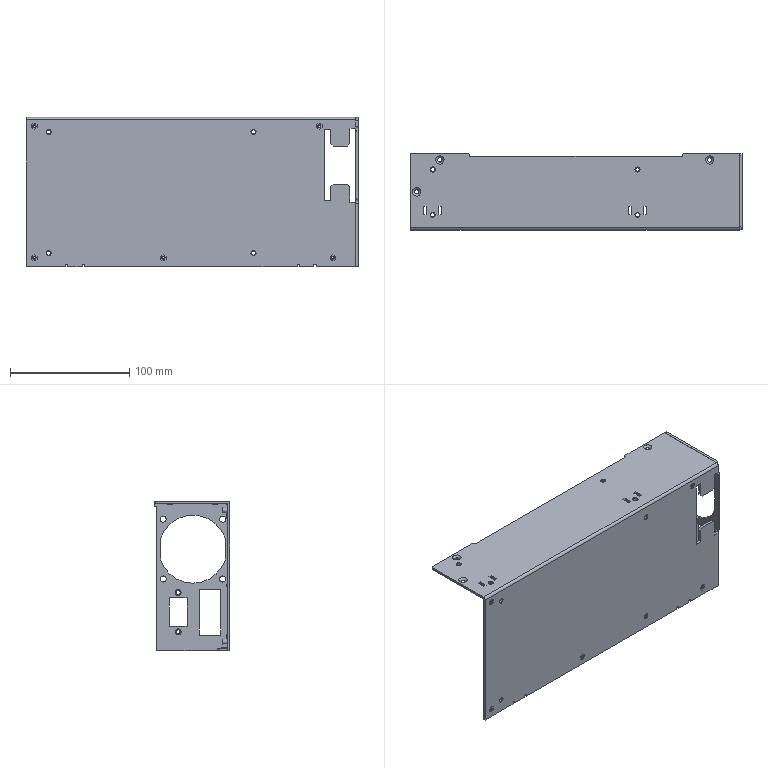Part | NX | features BREP 6 | 6 solids | 278 faces | box 278 x 63.5 x 125 mm | volume 107767 mm3 | plane 177 | cylinder 69 | torus 29 | cone 3 | commonest cylinder face diameters 2 x16 3.3 x10 4 x9 1.822 x5 3.2 x5 4.19 x5